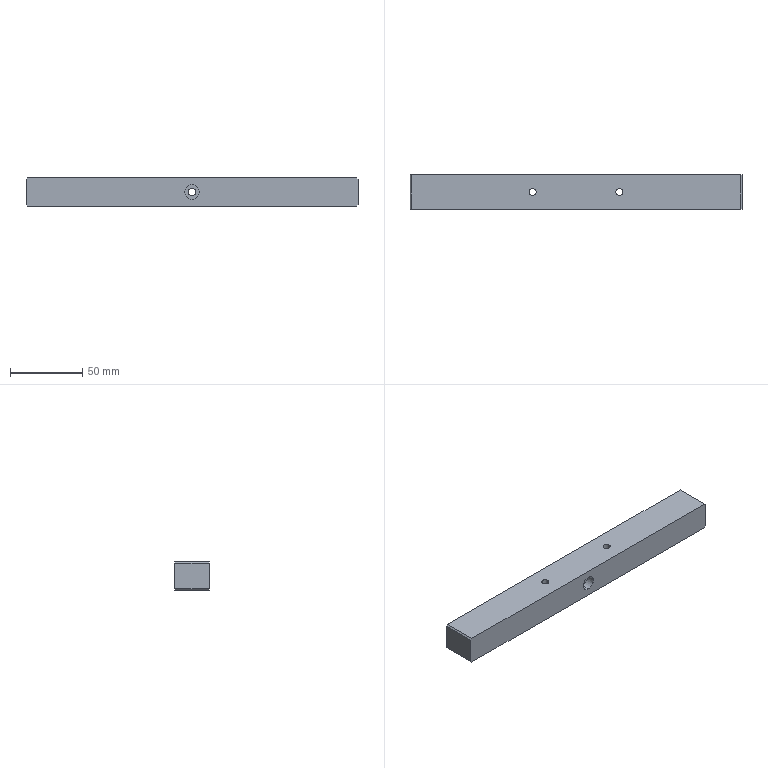Part | STEP file | A14-023 | 1 solid | 21 faces | box 230 x 24 x 20 mm | volume 108684 mm3 | plane 11 | cylinder 8 | cone 2 | commonest cylinder face diameters 5 x4 5.5 x2 10 x2